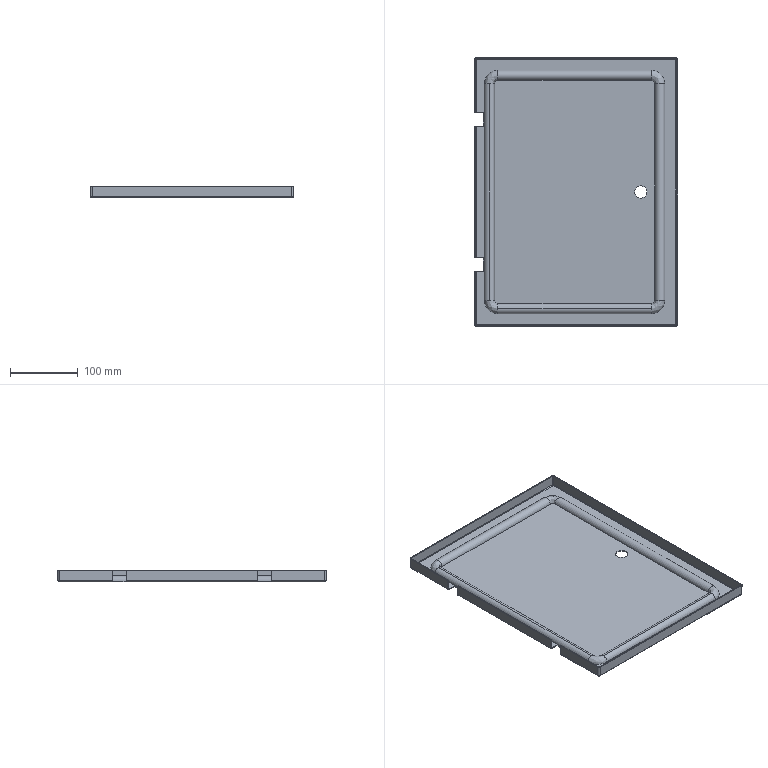Part | SolidWorks | features ICE 11, MoveFace 3, Fillet 2, BaseBody 1 | 1 solid | 63 faces | box 299.3 x 395 x 17.2 mm | volume 268537 mm3 | cylinder 28 | plane 23 | sphere 8 | spline 4 | commonest cylinder face diameters 2.4 x10 4.8 x10 15 x6 18 x2